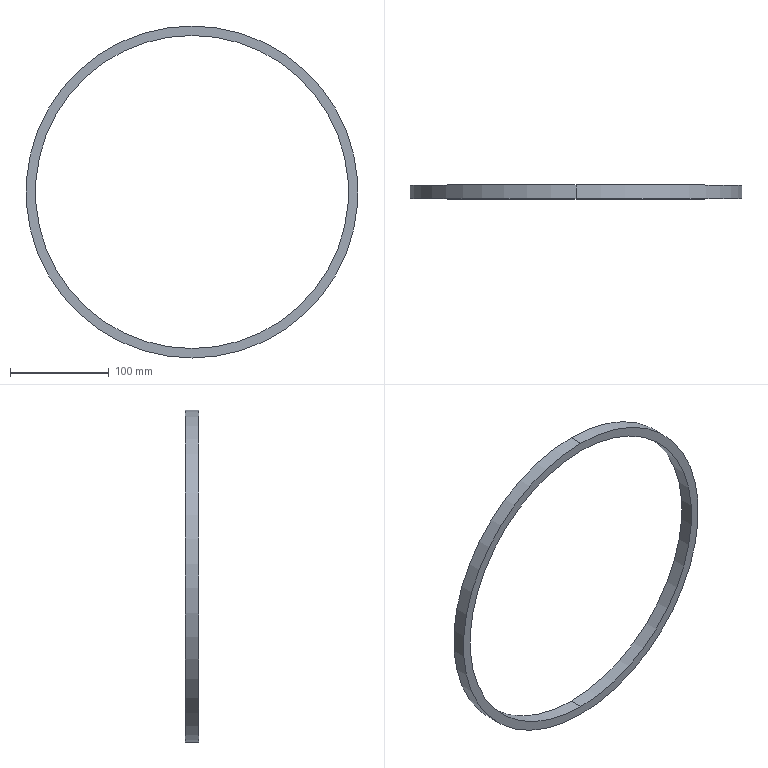Part | SolidWorks | features BaseBody 1, Scale 1 | 1 solid | 6 faces | box 336 x 13.8 x 336 mm | volume 135847 mm3 | cylinder 4 | plane 2 | commonest cylinder face diameters 316.8 x2 336 x2
STEP:
#1=CARTESIAN_POINT('',(0.,12.65,158.4));
#2=VERTEX_POINT('',#1);
#3=CARTESIAN_POINT('',(0.,12.65,-158.4));
#4=VERTEX_POINT('',#3);
#5=CARTESIAN_POINT('',(0.,12.65,0.));
#6=DIRECTION('',(0.,-1.,0.));
#7=DIRECTION('',(0.,0.,-1.));
#8=AXIS2_PLACEMENT_3D('',#5,#6,#7);
#9=CIRCLE('',#8,158.4);
#10=EDGE_CURVE('',#2,#4,#9,.T.);
#11=ORIENTED_EDGE('',*,*,#10,.F.);
#12=CARTESIAN_POINT('',(0.,-1.15,158.4));
#13=VERTEX_POINT('',#12);
#14=CARTESIAN_POINT('',(0.,12.65,158.4));
#15=DIRECTION('',(0.,-1.,0.));
#16=VECTOR('',#15,1000.);
#17=LINE('',#14,#16);
#18=EDGE_CURVE('',#2,#13,#17,.T.);
#19=ORIENTED_EDGE('',*,*,#18,.T.);
#20=CARTESIAN_POINT('',(0.,-1.15,-158.4));
#21=VERTEX_POINT('',#20);
#22=CARTESIAN_POINT('',(0.,-1.15,0.));
#23=DIRECTION('',(0.,1.,0.));
#24=DIRECTION('',(0.,0.,-1.));
#25=AXIS2_PLACEMENT_3D('',#22,#23,#24);
#26=CIRCLE('',#25,158.4);
#27=EDGE_CURVE('',#21,#13,#26,.T.);
#28=ORIENTED_EDGE('',*,*,#27,.F.);
#29=CARTESIAN_POINT('',(0.,12.65,-158.4));
#30=DIRECTION('',(0.,-1.,0.));
#31=VECTOR('',#30,1000.);
#32=LINE('',#29,#31);
#33=EDGE_CURVE('',#4,#21,#32,.T.);
#34=ORIENTED_EDGE('',*,*,#33,.F.);
#35=EDGE_LOOP('',(#11,#19,#28,#34));
#36=FACE_OUTER_BOUND('',#35,.T.);
#37=CARTESIAN_POINT('',(0.,12.65,0.));
#38=DIRECTION('',(0.,-1.,0.));
#39=DIRECTION('',(0.,0.,-1.));
#40=AXIS2_PLACEMENT_3D('',#37,#38,#39);
#41=CYLINDRICAL_SURFACE('',#40,158.4);
#42=ADVANCED_FACE('',(#36),#41,.F.);
#43=CARTESIAN_POINT('',(0.,12.65,168.));
#44=VERTEX_POINT('',#43);
#45=CARTESIAN_POINT('',(0.,12.65,-168.));
#46=VERTEX_POINT('',#45);
#47=CARTESIAN_POINT('',(0.,12.65,0.));
#48=DIRECTION('',(0.,1.,0.));
#49=DIRECTION('',(0.,0.,-1.));
#50=AXIS2_PLACEMENT_3D('',#47,#48,#49);
#51=CIRCLE('',#50,168.);
#52=EDGE_CURVE('',#44,#46,#51,.T.);
#53=ORIENTED_EDGE('',*,*,#52,.F.);
#54=CARTESIAN_POINT('',(0.,-1.15,168.));
#55=VERTEX_POINT('',#54);
#56=CARTESIAN_POINT('',(0.,12.65,168.));
#57=DIRECTION('',(0.,-1.,0.));
#58=VECTOR('',#57,1000.);
#59=LINE('',#56,#58);
#60=EDGE_CURVE('',#44,#55,#59,.T.);
#61=ORIENTED_EDGE('',*,*,#60,.T.);
#62=CARTESIAN_POINT('',(0.,-1.15,-168.));
#63=VERTEX_POINT('',#62);
#64=CARTESIAN_POINT('',(0.,-1.15,0.));
#65=DIRECTION('',(0.,1.,0.));
#66=DIRECTION('',(0.,0.,-1.));
#67=AXIS2_PLACEMENT_3D('',#64,#65,#66);
#68=CIRCLE('',#67,168.);
#69=EDGE_CURVE('',#55,#63,#68,.T.);
#70=ORIENTED_EDGE('',*,*,#69,.T.);
#71=CARTESIAN_POINT('',(0.,12.65,-168.));
#72=DIRECTION('',(0.,-1.,0.));
#73=VECTOR('',#72,1000.);
#74=LINE('',#71,#73);
#75=EDGE_CURVE('',#46,#63,#74,.T.);
#76=ORIENTED_EDGE('',*,*,#75,.F.);
#77=EDGE_LOOP('',(#53,#61,#70,#76));
#78=FACE_OUTER_BOUND('',#77,.T.);
#79=CARTESIAN_POINT('',(0.,12.65,0.));
#80=DIRECTION('',(0.,-1.,0.));
#81=DIRECTION('',(0.,0.,-1.));
#82=AXIS2_PLACEMENT_3D('',#79,#80,#81);
#83=CYLINDRICAL_SURFACE('',#82,168.);
#84=ADVANCED_FACE('',(#78),#83,.T.);
#85=CARTESIAN_POINT('',(0.,12.65,0.));
#86=DIRECTION('',(0.,-1.,0.));
#87=DIRECTION('',(0.,0.,-1.));
#88=AXIS2_PLACEMENT_3D('',#85,#86,#87);
#89=CIRCLE('',#88,158.4);
#90=EDGE_CURVE('',#4,#2,#89,.T.);
#91=ORIENTED_EDGE('',*,*,#90,.T.);
#92=ORIENTED_EDGE('',*,*,#10,.T.);
#93=EDGE_LOOP('',(#91,#92));
#94=FACE_BOUND('',#93,.T.);
#95=CARTESIAN_POINT('',(0.,12.65,0.));
#96=DIRECTION('',(0.,1.,0.));
#97=DIRECTION('',(0.,0.,-1.));
#98=AXIS2_PLACEMENT_3D('',#95,#96,#97);
#99=CIRCLE('',#98,168.);
#100=EDGE_CURVE('',#46,#44,#99,.T.);
#101=ORIENTED_EDGE('',*,*,#100,.T.);
#102=ORIENTED_EDGE('',*,*,#52,.T.);
#103=EDGE_LOOP('',(#101,#102));
#104=FACE_OUTER_BOUND('',#103,.T.);
#105=CARTESIAN_POINT('',(0.,12.65,0.));
#106=DIRECTION('',(0.,1.,0.));
#107=DIRECTION('',(0.,0.,1.));
#108=AXIS2_PLACEMENT_3D('',#105,#106,#107);
#109=PLANE('',#108);
#110=ADVANCED_FACE('',(#94,#104),#109,.T.);
#111=ORIENTED_EDGE('',*,*,#18,.F.);
#112=ORIENTED_EDGE('',*,*,#90,.F.);
#113=ORIENTED_EDGE('',*,*,#33,.T.);
#114=CARTESIAN_POINT('',(0.,-1.15,0.));
#115=DIRECTION('',(0.,1.,0.));
#116=DIRECTION('',(0.,0.,-1.));
#117=AXIS2_PLACEMENT_3D('',#114,#115,#116);
#118=CIRCLE('',#117,158.4);
#119=EDGE_CURVE('',#13,#21,#118,.T.);
#120=ORIENTED_EDGE('',*,*,#119,.F.);
#121=EDGE_LOOP('',(#111,#112,#113,#120));
#122=FACE_OUTER_BOUND('',#121,.T.);
#123=CARTESIAN_POINT('',(0.,12.65,0.));
#124=DIRECTION('',(0.,-1.,0.));
#125=DIRECTION('',(0.,0.,-1.));
#126=AXIS2_PLACEMENT_3D('',#123,#124,#125);
#127=CYLINDRICAL_SURFACE('',#126,158.4);
#128=ADVANCED_FACE('',(#122),#127,.F.);
#129=ORIENTED_EDGE('',*,*,#60,.F.);
#130=ORIENTED_EDGE('',*,*,#100,.F.);
#131=ORIENTED_EDGE('',*,*,#75,.T.);
#132=CARTESIAN_POINT('',(0.,-1.15,0.));
#133=DIRECTION('',(0.,1.,0.));
#134=DIRECTION('',(0.,0.,-1.));
#135=AXIS2_PLACEMENT_3D('',#132,#133,#134);
#136=CIRCLE('',#135,168.);
#137=EDGE_CURVE('',#63,#55,#136,.T.);
#138=ORIENTED_EDGE('',*,*,#137,.T.);
#139=EDGE_LOOP('',(#129,#130,#131,#138));
#140=FACE_OUTER_BOUND('',#139,.T.);
#141=CARTESIAN_POINT('',(0.,12.65,0.));
#142=DIRECTION('',(0.,-1.,0.));
#143=DIRECTION('',(0.,0.,-1.));
#144=AXIS2_PLACEMENT_3D('',#141,#142,#143);
#145=CYLINDRICAL_SURFACE('',#144,168.);
#146=ADVANCED_FACE('',(#140),#145,.T.);
#147=ORIENTED_EDGE('',*,*,#27,.T.);
#148=ORIENTED_EDGE('',*,*,#119,.T.);
#149=EDGE_LOOP('',(#147,#148));
#150=FACE_BOUND('',#149,.T.);
#151=ORIENTED_EDGE('',*,*,#137,.F.);
#152=ORIENTED_EDGE('',*,*,#69,.F.);
#153=EDGE_LOOP('',(#151,#152));
#154=FACE_OUTER_BOUND('',#153,.T.);
#155=CARTESIAN_POINT('',(0.,-1.15,0.));
#156=DIRECTION('',(0.,1.,0.));
#157=DIRECTION('',(0.,0.,1.));
#158=AXIS2_PLACEMENT_3D('',#155,#156,#157);
#159=PLANE('',#158);
#160=ADVANCED_FACE('',(#150,#154),#159,.F.);
#161=CLOSED_SHELL('',(#42,#84,#110,#128,#146,#160));
#162=MANIFOLD_SOLID_BREP('',#161);
#163=CARTESIAN_POINT('',(0.,0.,0.));
#164=DIRECTION('',(0.,0.,1.));
#165=DIRECTION('',(1.,0.,0.));
#166=AXIS2_PLACEMENT_3D('',#163,#164,#165);
#167=(LENGTH_UNIT()NAMED_UNIT(*)SI_UNIT(.MILLI.,.METRE.));
#168=UNCERTAINTY_MEASURE_WITH_UNIT(LENGTH_MEASURE(0.00001),#167,'','');
#169=(NAMED_UNIT(*)PLANE_ANGLE_UNIT()SI_UNIT($,.RADIAN.));
#170=(NAMED_UNIT(*)SI_UNIT($,.STERADIAN.)SOLID_ANGLE_UNIT());
#171=(GEOMETRIC_REPRESENTATION_CONTEXT(3)GLOBAL_UNCERTAINTY_ASSIGNED_CONTEXT((#168))GLOBAL_UNIT_ASSIGNED_CONTEXT((#167,#169,#170))REPRESENTATION_CONTEXT('',''));
#172=ADVANCED_BREP_SHAPE_REPRESENTATION('',(#162,#166),#171);